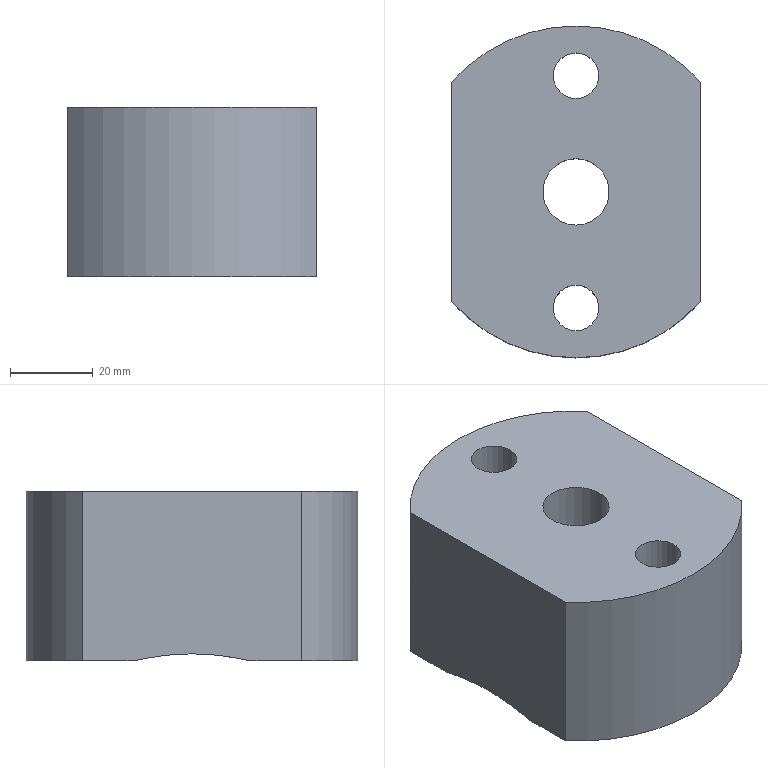Part | NX | features solid 2 | 1 solid | 17 faces | box 60 x 80 x 41 mm | volume 135787 mm3 | plane 8 | cylinder 8 | cone 1 | commonest cylinder face diameters 18 x3 11 x2 80 x2 16 x1
STEP:
#1=CARTESIAN_POINT('',(84.977,65.387,70.13));
#2=VERTEX_POINT('',#1);
#3=CARTESIAN_POINT('',(107.033,47.365,70.13));
#4=VERTEX_POINT('',#3);
#5=CARTESIAN_POINT('',(114.977,79.595,70.13));
#6=DIRECTION('',(0.,0.,-1.));
#7=DIRECTION('',(0.,-1.,0.));
#8=AXIS2_PLACEMENT_3D('',#5,#6,#7);
#9=CIRCLE('',#8,33.194);
#10=EDGE_CURVE('',#2,#4,#9,.F.);
#11=ORIENTED_EDGE('',*,*,#10,.T.);
#12=CARTESIAN_POINT('',(122.921,47.365,70.13));
#13=VERTEX_POINT('',#12);
#14=CARTESIAN_POINT('',(114.977,51.595,70.13));
#15=DIRECTION('',(0.,0.,-1.));
#16=DIRECTION('',(0.,-1.,0.));
#17=AXIS2_PLACEMENT_3D('',#14,#15,#16);
#18=CIRCLE('',#17,9.);
#19=EDGE_CURVE('',#4,#13,#18,.F.);
#20=ORIENTED_EDGE('',*,*,#19,.T.);
#21=CARTESIAN_POINT('',(144.977,65.387,70.13));
#22=VERTEX_POINT('',#21);
#23=CARTESIAN_POINT('',(114.977,79.595,70.13));
#24=DIRECTION('',(0.,0.,-1.));
#25=DIRECTION('',(0.,-1.,0.));
#26=AXIS2_PLACEMENT_3D('',#23,#24,#25);
#27=CIRCLE('',#26,33.194);
#28=EDGE_CURVE('',#13,#22,#27,.F.);
#29=ORIENTED_EDGE('',*,*,#28,.T.);
#30=CARTESIAN_POINT('',(144.977,53.138,70.13));
#31=VERTEX_POINT('',#30);
#32=CARTESIAN_POINT('',(144.977,79.595,70.13));
#33=DIRECTION('',(0.,1.,0.));
#34=VECTOR('',#33,1000.);
#35=LINE('',#32,#34);
#36=EDGE_CURVE('',#31,#22,#35,.T.);
#37=ORIENTED_EDGE('',*,*,#36,.F.);
#38=CARTESIAN_POINT('',(84.977,53.138,70.13));
#39=VERTEX_POINT('',#38);
#40=CARTESIAN_POINT('',(114.977,79.595,70.13));
#41=DIRECTION('',(0.,0.,-1.));
#42=DIRECTION('',(0.,-1.,0.));
#43=AXIS2_PLACEMENT_3D('',#40,#41,#42);
#44=CIRCLE('',#43,40.);
#45=EDGE_CURVE('',#31,#39,#44,.T.);
#46=ORIENTED_EDGE('',*,*,#45,.T.);
#47=CARTESIAN_POINT('',(84.977,79.595,70.13));
#48=DIRECTION('',(0.,-1.,0.));
#49=VECTOR('',#48,1000.);
#50=LINE('',#47,#49);
#51=EDGE_CURVE('',#2,#39,#50,.T.);
#52=ORIENTED_EDGE('',*,*,#51,.F.);
#53=EDGE_LOOP('',(#11,#20,#29,#37,#46,#52));
#54=FACE_BOUND('',#53,.T.);
#55=CARTESIAN_POINT('',(114.977,79.595,70.13));
#56=DIRECTION('',(0.,0.,1.));
#57=DIRECTION('',(0.,1.,0.));
#58=AXIS2_PLACEMENT_3D('',#55,#56,#57);
#59=PLANE('',#58);
#60=ADVANCED_FACE('',(#54),#59,.F.);
#61=CARTESIAN_POINT('',(84.977,106.053,70.13));
#62=VERTEX_POINT('',#61);
#63=CARTESIAN_POINT('',(144.977,106.053,70.13));
#64=VERTEX_POINT('',#63);
#65=CARTESIAN_POINT('',(114.977,79.595,70.13));
#66=DIRECTION('',(0.,0.,-1.));
#67=DIRECTION('',(0.,-1.,0.));
#68=AXIS2_PLACEMENT_3D('',#65,#66,#67);
#69=CIRCLE('',#68,40.);
#70=EDGE_CURVE('',#62,#64,#69,.T.);
#71=ORIENTED_EDGE('',*,*,#70,.T.);
#72=CARTESIAN_POINT('',(144.977,93.803,70.13));
#73=VERTEX_POINT('',#72);
#74=CARTESIAN_POINT('',(144.977,79.595,70.13));
#75=DIRECTION('',(0.,1.,0.));
#76=VECTOR('',#75,1000.);
#77=LINE('',#74,#76);
#78=EDGE_CURVE('',#73,#64,#77,.T.);
#79=ORIENTED_EDGE('',*,*,#78,.F.);
#80=CARTESIAN_POINT('',(122.921,111.825,70.13));
#81=VERTEX_POINT('',#80);
#82=CARTESIAN_POINT('',(114.977,79.595,70.13));
#83=DIRECTION('',(0.,0.,-1.));
#84=DIRECTION('',(0.,-1.,0.));
#85=AXIS2_PLACEMENT_3D('',#82,#83,#84);
#86=CIRCLE('',#85,33.194);
#87=EDGE_CURVE('',#73,#81,#86,.F.);
#88=ORIENTED_EDGE('',*,*,#87,.T.);
#89=CARTESIAN_POINT('',(107.033,111.825,70.13));
#90=VERTEX_POINT('',#89);
#91=CARTESIAN_POINT('',(114.977,107.595,70.13));
#92=DIRECTION('',(0.,0.,-1.));
#93=DIRECTION('',(0.,-1.,0.));
#94=AXIS2_PLACEMENT_3D('',#91,#92,#93);
#95=CIRCLE('',#94,9.);
#96=EDGE_CURVE('',#81,#90,#95,.F.);
#97=ORIENTED_EDGE('',*,*,#96,.T.);
#98=CARTESIAN_POINT('',(84.977,93.803,70.13));
#99=VERTEX_POINT('',#98);
#100=CARTESIAN_POINT('',(114.977,79.595,70.13));
#101=DIRECTION('',(0.,0.,-1.));
#102=DIRECTION('',(0.,-1.,0.));
#103=AXIS2_PLACEMENT_3D('',#100,#101,#102);
#104=CIRCLE('',#103,33.194);
#105=EDGE_CURVE('',#90,#99,#104,.F.);
#106=ORIENTED_EDGE('',*,*,#105,.T.);
#107=CARTESIAN_POINT('',(84.977,79.595,70.13));
#108=DIRECTION('',(0.,-1.,0.));
#109=VECTOR('',#108,1000.);
#110=LINE('',#107,#109);
#111=EDGE_CURVE('',#62,#99,#110,.T.);
#112=ORIENTED_EDGE('',*,*,#111,.F.);
#113=EDGE_LOOP('',(#71,#79,#88,#97,#106,#112));
#114=FACE_BOUND('',#113,.T.);
#115=CARTESIAN_POINT('',(114.977,79.595,70.13));
#116=DIRECTION('',(0.,0.,1.));
#117=DIRECTION('',(0.,1.,0.));
#118=AXIS2_PLACEMENT_3D('',#115,#116,#117);
#119=PLANE('',#118);
#120=ADVANCED_FACE('',(#114),#119,.F.);
#121=CARTESIAN_POINT('',(144.977,93.803,70.13));
#122=CARTESIAN_POINT('',(144.977,89.113,71.209));
#123=CARTESIAN_POINT('',(144.977,82.026,72.165));
#124=CARTESIAN_POINT('',(144.977,72.372,71.527));
#125=CARTESIAN_POINT('',(144.977,67.701,70.662));
#126=CARTESIAN_POINT('',(144.977,65.387,70.13));
#127=B_SPLINE_CURVE_WITH_KNOTS('',3,(#121,#122,#123,#124,#125,#126),.UNSPECIFIED.,.F.,.F.,(4,1,1,4),(0.03559,0.04991,0.05707,0.06423),.UNSPECIFIED.);
#128=EDGE_CURVE('',#73,#22,#127,.T.);
#129=ORIENTED_EDGE('',*,*,#128,.T.);
#130=ORIENTED_EDGE('',*,*,#28,.F.);
#131=CARTESIAN_POINT('',(122.921,47.365,70.13));
#132=CARTESIAN_POINT('',(123.662,48.757,70.761));
#133=CARTESIAN_POINT('',(124.348,51.796,72.208));
#134=CARTESIAN_POINT('',(123.14,56.181,74.638));
#135=CARTESIAN_POINT('',(119.985,59.581,76.93));
#136=CARTESIAN_POINT('',(115.018,61.095,78.165));
#137=CARTESIAN_POINT('',(110.,59.61,76.952));
#138=CARTESIAN_POINT('',(106.821,56.198,74.648));
#139=CARTESIAN_POINT('',(105.604,51.808,72.214));
#140=CARTESIAN_POINT('',(106.291,48.759,70.762));
#141=CARTESIAN_POINT('',(107.033,47.365,70.13));
#142=B_SPLINE_CURVE_WITH_KNOTS('',3,(#131,#132,#133,#134,#135,#136,#137,#138,#139,#140,#141),.UNSPECIFIED.,.F.,.F.,(4,1,1,1,1,1,1,1,4),(0.,0.005018,0.01004,0.01506,0.02007,0.02509,0.03011,0.03513,0.04015),.UNSPECIFIED.);
#143=EDGE_CURVE('',#13,#4,#142,.T.);
#144=ORIENTED_EDGE('',*,*,#143,.T.);
#145=ORIENTED_EDGE('',*,*,#10,.F.);
#146=CARTESIAN_POINT('',(84.977,65.387,70.13));
#147=CARTESIAN_POINT('',(84.977,70.077,71.209));
#148=CARTESIAN_POINT('',(84.977,77.164,72.165));
#149=CARTESIAN_POINT('',(84.977,86.818,71.527));
#150=CARTESIAN_POINT('',(84.977,91.49,70.662));
#151=CARTESIAN_POINT('',(84.977,93.803,70.13));
#152=B_SPLINE_CURVE_WITH_KNOTS('',3,(#146,#147,#148,#149,#150,#151),.UNSPECIFIED.,.F.,.F.,(4,1,1,4),(0.03559,0.04991,0.05707,0.06423),.UNSPECIFIED.);
#153=EDGE_CURVE('',#2,#99,#152,.T.);
#154=ORIENTED_EDGE('',*,*,#153,.T.);
#155=ORIENTED_EDGE('',*,*,#105,.F.);
#156=CARTESIAN_POINT('',(107.033,111.825,70.13));
#157=CARTESIAN_POINT('',(106.292,110.433,70.761));
#158=CARTESIAN_POINT('',(105.606,107.394,72.208));
#159=CARTESIAN_POINT('',(106.813,103.009,74.638));
#160=CARTESIAN_POINT('',(109.968,99.61,76.93));
#161=CARTESIAN_POINT('',(114.935,98.095,78.165));
#162=CARTESIAN_POINT('',(119.953,99.581,76.952));
#163=CARTESIAN_POINT('',(123.132,102.992,74.648));
#164=CARTESIAN_POINT('',(124.349,107.382,72.214));
#165=CARTESIAN_POINT('',(123.663,110.431,70.762));
#166=CARTESIAN_POINT('',(122.921,111.825,70.13));
#167=B_SPLINE_CURVE_WITH_KNOTS('',3,(#156,#157,#158,#159,#160,#161,#162,#163,#164,#165,#166),.UNSPECIFIED.,.F.,.F.,(4,1,1,1,1,1,1,1,4),(0.,0.005018,0.01004,0.01506,0.02007,0.02509,0.03011,0.03513,0.04015),.UNSPECIFIED.);
#168=EDGE_CURVE('',#90,#81,#167,.T.);
#169=ORIENTED_EDGE('',*,*,#168,.T.);
#170=ORIENTED_EDGE('',*,*,#87,.F.);
#171=EDGE_LOOP('',(#129,#130,#144,#145,#154,#155,#169,#170));
#172=FACE_BOUND('',#171,.T.);
#173=CARTESIAN_POINT('',(114.977,88.595,83.13));
#174=VERTEX_POINT('',#173);
#175=CARTESIAN_POINT('',(114.977,79.595,83.13));
#176=DIRECTION('',(0.,0.,1.));
#177=DIRECTION('',(0.,1.,0.));
#178=AXIS2_PLACEMENT_3D('',#175,#176,#177);
#179=CIRCLE('',#178,9.);
#180=EDGE_CURVE('',#174,#174,#179,.T.);
#181=ORIENTED_EDGE('',*,*,#180,.T.);
#182=EDGE_LOOP('',(#181));
#183=FACE_BOUND('',#182,.T.);
#184=CARTESIAN_POINT('',(114.977,79.595,83.13));
#185=DIRECTION('',(0.,0.,-1.));
#186=DIRECTION('',(0.,-1.,0.));
#187=AXIS2_PLACEMENT_3D('',#184,#185,#186);
#188=CONICAL_SURFACE('',#187,9.,1.078);
#189=ADVANCED_FACE('',(#172,#183),#188,.F.);
#190=CARTESIAN_POINT('',(114.977,71.595,111.13));
#191=VERTEX_POINT('',#190);
#192=CARTESIAN_POINT('',(114.977,79.595,111.13));
#193=DIRECTION('',(0.,0.,1.));
#194=DIRECTION('',(0.,-1.,0.));
#195=AXIS2_PLACEMENT_3D('',#192,#193,#194);
#196=CIRCLE('',#195,8.);
#197=EDGE_CURVE('',#191,#191,#196,.F.);
#198=ORIENTED_EDGE('',*,*,#197,.F.);
#199=EDGE_LOOP('',(#198));
#200=FACE_BOUND('',#199,.T.);
#201=CARTESIAN_POINT('',(114.977,87.595,86.13));
#202=VERTEX_POINT('',#201);
#203=CARTESIAN_POINT('',(114.977,79.595,86.13));
#204=DIRECTION('',(0.,0.,1.));
#205=DIRECTION('',(0.,1.,0.));
#206=AXIS2_PLACEMENT_3D('',#203,#204,#205);
#207=CIRCLE('',#206,8.);
#208=EDGE_CURVE('',#202,#202,#207,.T.);
#209=ORIENTED_EDGE('',*,*,#208,.F.);
#210=EDGE_LOOP('',(#209));
#211=FACE_BOUND('',#210,.T.);
#212=CARTESIAN_POINT('',(114.977,79.595,44.13));
#213=DIRECTION('',(0.,0.,1.));
#214=DIRECTION('',(0.,1.,0.));
#215=AXIS2_PLACEMENT_3D('',#212,#213,#214);
#216=CYLINDRICAL_SURFACE('',#215,8.);
#217=ADVANCED_FACE('',(#200,#211),#216,.F.);
#218=CARTESIAN_POINT('',(114.977,46.095,111.13));
#219=VERTEX_POINT('',#218);
#220=CARTESIAN_POINT('',(114.977,51.595,111.13));
#221=DIRECTION('',(0.,0.,1.));
#222=DIRECTION('',(0.,-1.,0.));
#223=AXIS2_PLACEMENT_3D('',#220,#221,#222);
#224=CIRCLE('',#223,5.5);
#225=EDGE_CURVE('',#219,#219,#224,.F.);
#226=ORIENTED_EDGE('',*,*,#225,.T.);
#227=EDGE_LOOP('',(#226));
#228=FACE_BOUND('',#227,.T.);
#229=CARTESIAN_POINT('',(84.977,53.138,111.13));
#230=VERTEX_POINT('',#229);
#231=CARTESIAN_POINT('',(144.977,53.138,111.13));
#232=VERTEX_POINT('',#231);
#233=CARTESIAN_POINT('',(114.977,79.595,111.13));
#234=DIRECTION('',(0.,0.,1.));
#235=DIRECTION('',(0.,1.,0.));
#236=AXIS2_PLACEMENT_3D('',#233,#234,#235);
#237=CIRCLE('',#236,40.);
#238=EDGE_CURVE('',#230,#232,#237,.T.);
#239=ORIENTED_EDGE('',*,*,#238,.T.);
#240=CARTESIAN_POINT('',(144.977,106.053,111.13));
#241=VERTEX_POINT('',#240);
#242=CARTESIAN_POINT('',(144.977,79.595,111.13));
#243=DIRECTION('',(0.,-1.,0.));
#244=VECTOR('',#243,1000.);
#245=LINE('',#242,#244);
#246=EDGE_CURVE('',#241,#232,#245,.T.);
#247=ORIENTED_EDGE('',*,*,#246,.F.);
#248=CARTESIAN_POINT('',(84.977,106.053,111.13));
#249=VERTEX_POINT('',#248);
#250=CARTESIAN_POINT('',(114.977,79.595,111.13));
#251=DIRECTION('',(0.,0.,1.));
#252=DIRECTION('',(0.,1.,0.));
#253=AXIS2_PLACEMENT_3D('',#250,#251,#252);
#254=CIRCLE('',#253,40.);
#255=EDGE_CURVE('',#241,#249,#254,.T.);
#256=ORIENTED_EDGE('',*,*,#255,.T.);
#257=CARTESIAN_POINT('',(84.977,79.595,111.13));
#258=DIRECTION('',(0.,1.,0.));
#259=VECTOR('',#258,1000.);
#260=LINE('',#257,#259);
#261=EDGE_CURVE('',#230,#249,#260,.T.);
#262=ORIENTED_EDGE('',*,*,#261,.F.);
#263=EDGE_LOOP('',(#239,#247,#256,#262));
#264=FACE_BOUND('',#263,.T.);
#265=ORIENTED_EDGE('',*,*,#197,.T.);
#266=EDGE_LOOP('',(#265));
#267=FACE_BOUND('',#266,.T.);
#268=CARTESIAN_POINT('',(114.977,102.095,111.13));
#269=VERTEX_POINT('',#268);
#270=CARTESIAN_POINT('',(114.977,107.595,111.13));
#271=DIRECTION('',(0.,0.,1.));
#272=DIRECTION('',(0.,-1.,0.));
#273=AXIS2_PLACEMENT_3D('',#270,#271,#272);
#274=CIRCLE('',#273,5.5);
#275=EDGE_CURVE('',#269,#269,#274,.F.);
#276=ORIENTED_EDGE('',*,*,#275,.T.);
#277=EDGE_LOOP('',(#276));
#278=FACE_BOUND('',#277,.T.);
#279=CARTESIAN_POINT('',(114.977,79.595,111.13));
#280=DIRECTION('',(0.,0.,-1.));
#281=DIRECTION('',(0.,-1.,0.));
#282=AXIS2_PLACEMENT_3D('',#279,#280,#281);
#283=PLANE('',#282);
#284=ADVANCED_FACE('',(#228,#264,#267,#278),#283,.F.);
#285=ORIENTED_EDGE('',*,*,#45,.F.);
#286=CARTESIAN_POINT('',(144.977,53.138,36.13));
#287=DIRECTION('',(0.,0.,1.));
#288=VECTOR('',#287,1000.);
#289=LINE('',#286,#288);
#290=EDGE_CURVE('',#232,#31,#289,.F.);
#291=ORIENTED_EDGE('',*,*,#290,.F.);
#292=ORIENTED_EDGE('',*,*,#238,.F.);
#293=CARTESIAN_POINT('',(84.977,53.138,70.13));
#294=DIRECTION('',(0.,0.,1.));
#295=VECTOR('',#294,1000.);
#296=LINE('',#293,#295);
#297=EDGE_CURVE('',#39,#230,#296,.T.);
#298=ORIENTED_EDGE('',*,*,#297,.F.);
#299=EDGE_LOOP('',(#285,#291,#292,#298));
#300=FACE_BOUND('',#299,.T.);
#301=CARTESIAN_POINT('',(114.977,79.595,36.13));
#302=DIRECTION('',(0.,0.,1.));
#303=DIRECTION('',(0.,1.,0.));
#304=AXIS2_PLACEMENT_3D('',#301,#302,#303);
#305=CYLINDRICAL_SURFACE('',#304,40.);
#306=ADVANCED_FACE('',(#300),#305,.T.);
#307=ORIENTED_EDGE('',*,*,#255,.F.);
#308=CARTESIAN_POINT('',(144.977,106.053,36.13));
#309=DIRECTION('',(0.,0.,1.));
#310=VECTOR('',#309,1000.);
#311=LINE('',#308,#310);
#312=EDGE_CURVE('',#64,#241,#311,.T.);
#313=ORIENTED_EDGE('',*,*,#312,.F.);
#314=ORIENTED_EDGE('',*,*,#70,.F.);
#315=CARTESIAN_POINT('',(84.977,106.053,111.13));
#316=DIRECTION('',(0.,0.,1.));
#317=VECTOR('',#316,1000.);
#318=LINE('',#315,#317);
#319=EDGE_CURVE('',#249,#62,#318,.F.);
#320=ORIENTED_EDGE('',*,*,#319,.F.);
#321=EDGE_LOOP('',(#307,#313,#314,#320));
#322=FACE_BOUND('',#321,.T.);
#323=CARTESIAN_POINT('',(114.977,79.595,36.13));
#324=DIRECTION('',(0.,0.,1.));
#325=DIRECTION('',(0.,1.,0.));
#326=AXIS2_PLACEMENT_3D('',#323,#324,#325);
#327=CYLINDRICAL_SURFACE('',#326,40.);
#328=ADVANCED_FACE('',(#322),#327,.T.);
#329=ORIENTED_EDGE('',*,*,#78,.T.);
#330=ORIENTED_EDGE('',*,*,#312,.T.);
#331=ORIENTED_EDGE('',*,*,#246,.T.);
#332=ORIENTED_EDGE('',*,*,#290,.T.);
#333=ORIENTED_EDGE('',*,*,#36,.T.);
#334=ORIENTED_EDGE('',*,*,#128,.F.);
#335=EDGE_LOOP('',(#329,#330,#331,#332,#333,#334));
#336=FACE_BOUND('',#335,.T.);
#337=CARTESIAN_POINT('',(144.977,79.595,59.117));
#338=DIRECTION('',(-1.,0.,0.));
#339=DIRECTION('',(0.,0.,1.));
#340=AXIS2_PLACEMENT_3D('',#337,#338,#339);
#341=PLANE('',#340);
#342=ADVANCED_FACE('',(#336),#341,.F.);
#343=ORIENTED_EDGE('',*,*,#51,.T.);
#344=ORIENTED_EDGE('',*,*,#297,.T.);
#345=ORIENTED_EDGE('',*,*,#261,.T.);
#346=ORIENTED_EDGE('',*,*,#319,.T.);
#347=ORIENTED_EDGE('',*,*,#111,.T.);
#348=ORIENTED_EDGE('',*,*,#153,.F.);
#349=EDGE_LOOP('',(#343,#344,#345,#346,#347,#348));
#350=FACE_BOUND('',#349,.T.);
#351=CARTESIAN_POINT('',(84.977,79.595,59.117));
#352=DIRECTION('',(1.,0.,0.));
#353=DIRECTION('',(0.,0.,-1.));
#354=AXIS2_PLACEMENT_3D('',#351,#352,#353);
#355=PLANE('',#354);
#356=ADVANCED_FACE('',(#350),#355,.F.);
#357=CARTESIAN_POINT('',(114.977,46.095,96.13));
#358=VERTEX_POINT('',#357);
#359=CARTESIAN_POINT('',(114.977,51.595,96.13));
#360=DIRECTION('',(0.,0.,1.));
#361=DIRECTION('',(0.,-1.,0.));
#362=AXIS2_PLACEMENT_3D('',#359,#360,#361);
#363=CIRCLE('',#362,5.5);
#364=EDGE_CURVE('',#358,#358,#363,.F.);
#365=ORIENTED_EDGE('',*,*,#364,.T.);
#366=EDGE_LOOP('',(#365));
#367=FACE_BOUND('',#366,.T.);
#368=ORIENTED_EDGE('',*,*,#225,.F.);
#369=EDGE_LOOP('',(#368));
#370=FACE_BOUND('',#369,.T.);
#371=CARTESIAN_POINT('',(114.977,51.595,61.667));
#372=DIRECTION('',(0.,0.,1.));
#373=DIRECTION('',(0.,1.,0.));
#374=AXIS2_PLACEMENT_3D('',#371,#372,#373);
#375=CYLINDRICAL_SURFACE('',#374,5.5);
#376=ADVANCED_FACE('',(#367,#370),#375,.F.);
#377=CARTESIAN_POINT('',(114.977,42.595,96.13));
#378=VERTEX_POINT('',#377);
#379=CARTESIAN_POINT('',(114.977,51.595,96.13));
#380=DIRECTION('',(0.,0.,1.));
#381=DIRECTION('',(0.,-1.,0.));
#382=AXIS2_PLACEMENT_3D('',#379,#380,#381);
#383=CIRCLE('',#382,9.);
#384=EDGE_CURVE('',#378,#378,#383,.F.);
#385=ORIENTED_EDGE('',*,*,#384,.F.);
#386=EDGE_LOOP('',(#385));
#387=FACE_BOUND('',#386,.T.);
#388=ORIENTED_EDGE('',*,*,#19,.F.);
#389=ORIENTED_EDGE('',*,*,#143,.F.);
#390=EDGE_LOOP('',(#388,#389));
#391=FACE_BOUND('',#390,.T.);
#392=CARTESIAN_POINT('',(114.977,51.595,78.667));
#393=DIRECTION('',(0.,0.,-1.));
#394=DIRECTION('',(0.,-1.,0.));
#395=AXIS2_PLACEMENT_3D('',#392,#393,#394);
#396=CYLINDRICAL_SURFACE('',#395,9.);
#397=ADVANCED_FACE('',(#387,#391),#396,.F.);
#398=ORIENTED_EDGE('',*,*,#384,.T.);
#399=EDGE_LOOP('',(#398));
#400=FACE_BOUND('',#399,.T.);
#401=ORIENTED_EDGE('',*,*,#364,.F.);
#402=EDGE_LOOP('',(#401));
#403=FACE_BOUND('',#402,.T.);
#404=CARTESIAN_POINT('',(114.977,79.595,96.13));
#405=DIRECTION('',(0.,0.,-1.));
#406=DIRECTION('',(0.,-1.,0.));
#407=AXIS2_PLACEMENT_3D('',#404,#405,#406);
#408=PLANE('',#407);
#409=ADVANCED_FACE('',(#400,#403),#408,.T.);
#410=CARTESIAN_POINT('',(114.977,102.095,96.13));
#411=VERTEX_POINT('',#410);
#412=CARTESIAN_POINT('',(114.977,107.595,96.13));
#413=DIRECTION('',(0.,0.,1.));
#414=DIRECTION('',(0.,-1.,0.));
#415=AXIS2_PLACEMENT_3D('',#412,#413,#414);
#416=CIRCLE('',#415,5.5);
#417=EDGE_CURVE('',#411,#411,#416,.T.);
#418=ORIENTED_EDGE('',*,*,#417,.F.);
#419=EDGE_LOOP('',(#418));
#420=FACE_BOUND('',#419,.T.);
#421=ORIENTED_EDGE('',*,*,#275,.F.);
#422=EDGE_LOOP('',(#421));
#423=FACE_BOUND('',#422,.T.);
#424=CARTESIAN_POINT('',(114.977,107.595,61.667));
#425=DIRECTION('',(0.,0.,1.));
#426=DIRECTION('',(0.,1.,0.));
#427=AXIS2_PLACEMENT_3D('',#424,#425,#426);
#428=CYLINDRICAL_SURFACE('',#427,5.5);
#429=ADVANCED_FACE('',(#420,#423),#428,.F.);
#430=CARTESIAN_POINT('',(114.977,98.595,96.13));
#431=VERTEX_POINT('',#430);
#432=CARTESIAN_POINT('',(114.977,107.595,96.13));
#433=DIRECTION('',(0.,0.,1.));
#434=DIRECTION('',(0.,-1.,0.));
#435=AXIS2_PLACEMENT_3D('',#432,#433,#434);
#436=CIRCLE('',#435,9.);
#437=EDGE_CURVE('',#431,#431,#436,.F.);
#438=ORIENTED_EDGE('',*,*,#437,.F.);
#439=EDGE_LOOP('',(#438));
#440=FACE_BOUND('',#439,.T.);
#441=ORIENTED_EDGE('',*,*,#96,.F.);
#442=ORIENTED_EDGE('',*,*,#168,.F.);
#443=EDGE_LOOP('',(#441,#442));
#444=FACE_BOUND('',#443,.T.);
#445=CARTESIAN_POINT('',(114.977,107.595,78.667));
#446=DIRECTION('',(0.,0.,-1.));
#447=DIRECTION('',(0.,-1.,0.));
#448=AXIS2_PLACEMENT_3D('',#445,#446,#447);
#449=CYLINDRICAL_SURFACE('',#448,9.);
#450=ADVANCED_FACE('',(#440,#444),#449,.F.);
#451=ORIENTED_EDGE('',*,*,#437,.T.);
#452=EDGE_LOOP('',(#451));
#453=FACE_BOUND('',#452,.T.);
#454=ORIENTED_EDGE('',*,*,#417,.T.);
#455=EDGE_LOOP('',(#454));
#456=FACE_BOUND('',#455,.T.);
#457=CARTESIAN_POINT('',(114.977,79.595,96.13));
#458=DIRECTION('',(0.,0.,-1.));
#459=DIRECTION('',(0.,-1.,0.));
#460=AXIS2_PLACEMENT_3D('',#457,#458,#459);
#461=PLANE('',#460);
#462=ADVANCED_FACE('',(#453,#456),#461,.T.);
#463=CARTESIAN_POINT('',(114.977,88.595,86.13));
#464=VERTEX_POINT('',#463);
#465=CARTESIAN_POINT('',(114.977,79.595,86.13));
#466=DIRECTION('',(0.,0.,1.));
#467=DIRECTION('',(0.,1.,0.));
#468=AXIS2_PLACEMENT_3D('',#465,#466,#467);
#469=CIRCLE('',#468,9.);
#470=EDGE_CURVE('',#464,#464,#469,.T.);
#471=ORIENTED_EDGE('',*,*,#470,.T.);
#472=EDGE_LOOP('',(#471));
#473=FACE_BOUND('',#472,.T.);
#474=ORIENTED_EDGE('',*,*,#180,.F.);
#475=EDGE_LOOP('',(#474));
#476=FACE_BOUND('',#475,.T.);
#477=CARTESIAN_POINT('',(114.977,79.595,61.13));
#478=DIRECTION('',(0.,0.,1.));
#479=DIRECTION('',(0.,-1.,0.));
#480=AXIS2_PLACEMENT_3D('',#477,#478,#479);
#481=CYLINDRICAL_SURFACE('',#480,9.);
#482=ADVANCED_FACE('',(#473,#476),#481,.F.);
#483=ORIENTED_EDGE('',*,*,#208,.T.);
#484=EDGE_LOOP('',(#483));
#485=FACE_BOUND('',#484,.T.);
#486=ORIENTED_EDGE('',*,*,#470,.F.);
#487=EDGE_LOOP('',(#486));
#488=FACE_BOUND('',#487,.T.);
#489=CARTESIAN_POINT('',(114.977,79.595,86.13));
#490=DIRECTION('',(0.,0.,-1.));
#491=DIRECTION('',(0.,1.,0.));
#492=AXIS2_PLACEMENT_3D('',#489,#490,#491);
#493=PLANE('',#492);
#494=ADVANCED_FACE('',(#485,#488),#493,.T.);
#495=CLOSED_SHELL('',(#60,#120,#189,#217,#284,#306,#328,#342,#356,#376,#397,#409,#429,#450,#462,#482,#494));
#496=MANIFOLD_SOLID_BREP('',#495);
#497=(LENGTH_UNIT()NAMED_UNIT(*)SI_UNIT(.MILLI.,.METRE.));
#498=UNCERTAINTY_MEASURE_WITH_UNIT(LENGTH_MEASURE(0.0508),#497,'','');
#499=(NAMED_UNIT(*)PLANE_ANGLE_UNIT()SI_UNIT($,.RADIAN.));
#500=(NAMED_UNIT(*)SI_UNIT($,.STERADIAN.)SOLID_ANGLE_UNIT());
#501=(GEOMETRIC_REPRESENTATION_CONTEXT(3)GLOBAL_UNCERTAINTY_ASSIGNED_CONTEXT((#498))GLOBAL_UNIT_ASSIGNED_CONTEXT((#497,#499,#500))REPRESENTATION_CONTEXT('',''));
#502=ADVANCED_BREP_SHAPE_REPRESENTATION('',(#496),#501);